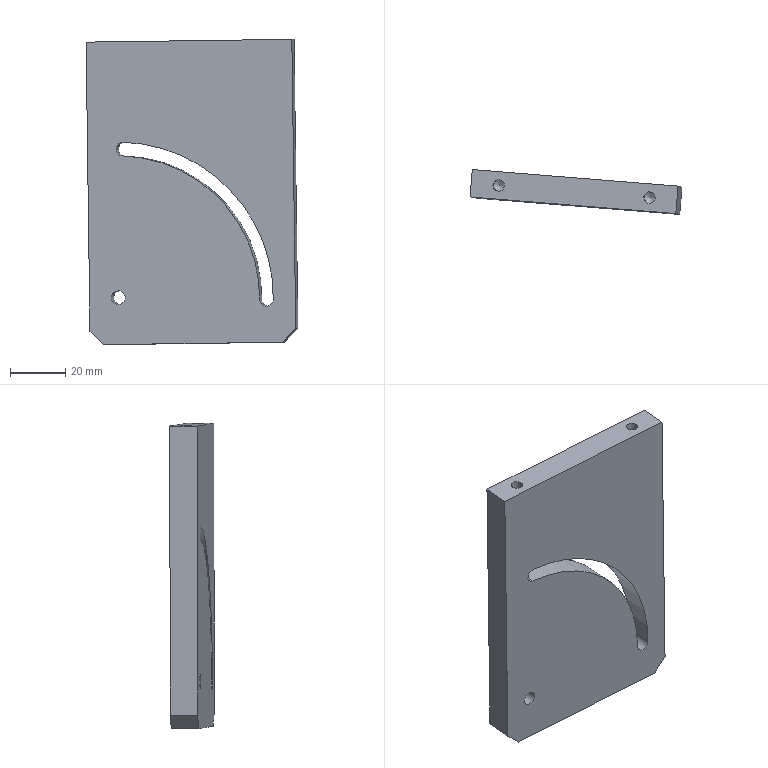Part | NX | 1 solid | 17 faces | box 76.959 x 16.139 x 110.936 mm | volume 77285 mm3 | plane 8 | cylinder 7 | cone 2 | commonest cylinder face diameters 5 x3 4.134 x2 103 x1 113 x1
STEP:
#1=CARTESIAN_POINT('',(751.636,682.46,909.631));
#2=VERTEX_POINT('',#1);
#3=CARTESIAN_POINT('',(752.438,692.427,909.627));
#4=VERTEX_POINT('',#3);
#5=CARTESIAN_POINT('',(751.636,682.46,909.631));
#6=DIRECTION('',(0.08022,0.9968,-0.0004004));
#7=VECTOR('',#6,1000.);
#8=LINE('',#5,#7);
#9=EDGE_CURVE('',#2,#4,#8,.T.);
#10=ORIENTED_EDGE('',*,*,#9,.F.);
#11=CARTESIAN_POINT('',(801.279,678.443,857.624));
#12=VERTEX_POINT('',#11);
#13=CARTESIAN_POINT('',(749.948,682.575,858.159));
#14=DIRECTION('',(-0.08022,-0.9968,0.0004004));
#15=DIRECTION('',(-0.01339,0.001479,0.9999));
#16=AXIS2_PLACEMENT_3D('',#13,#14,#15);
#17=CIRCLE('',#16,51.5);
#18=EDGE_CURVE('',#12,#2,#17,.T.);
#19=ORIENTED_EDGE('',*,*,#18,.F.);
#20=CARTESIAN_POINT('',(802.081,688.411,857.62));
#21=VERTEX_POINT('',#20);
#22=CARTESIAN_POINT('',(801.279,678.443,857.624));
#23=DIRECTION('',(-0.08022,-0.9968,0.0004004));
#24=VECTOR('',#23,1000.);
#25=LINE('',#22,#24);
#26=EDGE_CURVE('',#21,#12,#25,.T.);
#27=ORIENTED_EDGE('',*,*,#26,.F.);
#28=CARTESIAN_POINT('',(750.75,692.543,858.155));
#29=DIRECTION('',(0.08022,0.9968,-0.0004004));
#30=DIRECTION('',(-0.01339,0.001479,0.9999));
#31=AXIS2_PLACEMENT_3D('',#28,#29,#30);
#32=CIRCLE('',#31,51.5);
#33=EDGE_CURVE('',#4,#21,#32,.T.);
#34=ORIENTED_EDGE('',*,*,#33,.F.);
#35=EDGE_LOOP('',(#10,#19,#27,#34));
#36=FACE_BOUND('',#35,.T.);
#37=CARTESIAN_POINT('',(749.948,682.575,858.159));
#38=DIRECTION('',(0.08022,0.9968,-0.0004004));
#39=DIRECTION('',(-0.01339,0.001479,0.9999));
#40=AXIS2_PLACEMENT_3D('',#37,#38,#39);
#41=CYLINDRICAL_SURFACE('',#40,51.5);
#42=ADVANCED_FACE('',(#36),#41,.T.);
#43=CARTESIAN_POINT('',(751.8,682.449,914.628));
#44=VERTEX_POINT('',#43);
#45=CARTESIAN_POINT('',(751.718,682.454,912.13));
#46=DIRECTION('',(-0.08022,-0.9968,0.0004004));
#47=DIRECTION('',(-0.6979,0.05646,0.7139));
#48=AXIS2_PLACEMENT_3D('',#45,#46,#47);
#49=CIRCLE('',#48,2.5);
#50=EDGE_CURVE('',#44,#2,#49,.T.);
#51=ORIENTED_EDGE('',*,*,#50,.T.);
#52=ORIENTED_EDGE('',*,*,#9,.T.);
#53=CARTESIAN_POINT('',(752.602,692.416,914.624));
#54=VERTEX_POINT('',#53);
#55=CARTESIAN_POINT('',(752.52,692.422,912.126));
#56=DIRECTION('',(0.08022,0.9968,-0.0004004));
#57=DIRECTION('',(-0.7117,0.057,-0.7002));
#58=AXIS2_PLACEMENT_3D('',#55,#56,#57);
#59=CIRCLE('',#58,2.5);
#60=EDGE_CURVE('',#4,#54,#59,.T.);
#61=ORIENTED_EDGE('',*,*,#60,.T.);
#62=CARTESIAN_POINT('',(751.8,682.449,914.628));
#63=DIRECTION('',(-0.08022,-0.9968,0.0004004));
#64=VECTOR('',#63,1000.);
#65=LINE('',#62,#64);
#66=EDGE_CURVE('',#54,#44,#65,.T.);
#67=ORIENTED_EDGE('',*,*,#66,.T.);
#68=EDGE_LOOP('',(#51,#52,#61,#67));
#69=FACE_BOUND('',#68,.T.);
#70=CARTESIAN_POINT('',(751.718,682.454,912.13));
#71=DIRECTION('',(0.08022,0.9968,-0.0004004));
#72=DIRECTION('',(-0.6979,0.05646,0.7139));
#73=AXIS2_PLACEMENT_3D('',#70,#71,#72);
#74=CYLINDRICAL_SURFACE('',#73,2.5);
#75=ADVANCED_FACE('',(#69),#74,.F.);
#76=CARTESIAN_POINT('',(806.262,678.042,857.573));
#77=VERTEX_POINT('',#76);
#78=CARTESIAN_POINT('',(803.771,678.243,857.598));
#79=DIRECTION('',(-0.08022,-0.9968,0.0004004));
#80=DIRECTION('',(-0.7281,0.05832,-0.683));
#81=AXIS2_PLACEMENT_3D('',#78,#79,#80);
#82=CIRCLE('',#81,2.5);
#83=EDGE_CURVE('',#12,#77,#82,.T.);
#84=ORIENTED_EDGE('',*,*,#83,.T.);
#85=CARTESIAN_POINT('',(807.065,688.01,857.569));
#86=VERTEX_POINT('',#85);
#87=CARTESIAN_POINT('',(806.262,678.042,857.573));
#88=DIRECTION('',(0.08022,0.9968,-0.0004004));
#89=VECTOR('',#88,1000.);
#90=LINE('',#87,#89);
#91=EDGE_CURVE('',#77,#86,#90,.T.);
#92=ORIENTED_EDGE('',*,*,#91,.T.);
#93=CARTESIAN_POINT('',(804.573,688.211,857.594));
#94=DIRECTION('',(0.08022,0.9968,-0.0004004));
#95=DIRECTION('',(0.6808,-0.05509,-0.7304));
#96=AXIS2_PLACEMENT_3D('',#93,#94,#95);
#97=CIRCLE('',#96,2.5);
#98=EDGE_CURVE('',#86,#21,#97,.T.);
#99=ORIENTED_EDGE('',*,*,#98,.T.);
#100=ORIENTED_EDGE('',*,*,#26,.T.);
#101=EDGE_LOOP('',(#84,#92,#99,#100));
#102=FACE_BOUND('',#101,.T.);
#103=CARTESIAN_POINT('',(803.771,678.243,857.598));
#104=DIRECTION('',(0.08022,0.9968,-0.0004004));
#105=DIRECTION('',(0.6808,-0.05509,-0.7304));
#106=AXIS2_PLACEMENT_3D('',#103,#104,#105);
#107=CYLINDRICAL_SURFACE('',#106,2.5);
#108=ADVANCED_FACE('',(#102),#107,.F.);
#109=ORIENTED_EDGE('',*,*,#66,.F.);
#110=CARTESIAN_POINT('',(750.75,692.543,858.155));
#111=DIRECTION('',(-0.08022,-0.9968,0.0004004));
#112=DIRECTION('',(0.01339,-0.001479,-0.9999));
#113=AXIS2_PLACEMENT_3D('',#110,#111,#112);
#114=CIRCLE('',#113,56.5);
#115=EDGE_CURVE('',#86,#54,#114,.T.);
#116=ORIENTED_EDGE('',*,*,#115,.F.);
#117=ORIENTED_EDGE('',*,*,#91,.F.);
#118=CARTESIAN_POINT('',(749.948,682.575,858.159));
#119=DIRECTION('',(0.08022,0.9968,-0.0004004));
#120=DIRECTION('',(0.01339,-0.001479,-0.9999));
#121=AXIS2_PLACEMENT_3D('',#118,#119,#120);
#122=CIRCLE('',#121,56.5);
#123=EDGE_CURVE('',#44,#77,#122,.T.);
#124=ORIENTED_EDGE('',*,*,#123,.F.);
#125=EDGE_LOOP('',(#109,#116,#117,#124));
#126=FACE_BOUND('',#125,.T.);
#127=CARTESIAN_POINT('',(749.948,682.575,858.159));
#128=DIRECTION('',(0.08022,0.9968,-0.0004004));
#129=DIRECTION('',(0.01339,-0.001479,-0.9999));
#130=AXIS2_PLACEMENT_3D('',#127,#128,#129);
#131=CYLINDRICAL_SURFACE('',#130,56.5);
#132=ADVANCED_FACE('',(#126),#131,.F.);
#133=CARTESIAN_POINT('',(803.63,683.302,936.442));
#134=VERTEX_POINT('',#133);
#135=VERTEX_LOOP('',#134);
#136=FACE_BOUND('',#135,.T.);
#137=CARTESIAN_POINT('',(803.447,681.243,937.684));
#138=VERTEX_POINT('',#137);
#139=CARTESIAN_POINT('',(803.613,683.304,937.683));
#140=DIRECTION('',(-0.01339,0.001479,0.9999));
#141=DIRECTION('',(-0.08022,-0.9968,0.0004004));
#142=AXIS2_PLACEMENT_3D('',#139,#140,#141);
#143=CIRCLE('',#142,2.067);
#144=EDGE_CURVE('',#138,#138,#143,.T.);
#145=ORIENTED_EDGE('',*,*,#144,.T.);
#146=EDGE_LOOP('',(#145));
#147=FACE_BOUND('',#146,.T.);
#148=CARTESIAN_POINT('',(803.622,683.303,937.062));
#149=DIRECTION('',(-0.01339,0.001479,0.9999));
#150=DIRECTION('',(-0.08022,-0.9968,0.0004004));
#151=AXIS2_PLACEMENT_3D('',#148,#149,#150);
#152=CONICAL_SURFACE('',#151,1.034,1.03);
#153=ADVANCED_FACE('',(#136,#147),#152,.F.);
#154=ORIENTED_EDGE('',*,*,#144,.F.);
#155=EDGE_LOOP('',(#154));
#156=FACE_BOUND('',#155,.T.);
#157=CARTESIAN_POINT('',(803.257,681.264,951.883));
#158=VERTEX_POINT('',#157);
#159=CARTESIAN_POINT('',(803.423,683.325,951.882));
#160=DIRECTION('',(0.01339,-0.001479,-0.9999));
#161=DIRECTION('',(-0.08022,-0.9968,0.0004004));
#162=AXIS2_PLACEMENT_3D('',#159,#160,#161);
#163=CIRCLE('',#162,2.067);
#164=EDGE_CURVE('',#158,#158,#163,.T.);
#165=ORIENTED_EDGE('',*,*,#164,.F.);
#166=EDGE_LOOP('',(#165));
#167=FACE_BOUND('',#166,.T.);
#168=CARTESIAN_POINT('',(803.518,683.314,944.783));
#169=DIRECTION('',(-0.01339,0.001479,0.9999));
#170=DIRECTION('',(-0.08022,-0.9968,0.0004004));
#171=AXIS2_PLACEMENT_3D('',#168,#169,#170);
#172=CYLINDRICAL_SURFACE('',#171,2.067);
#173=ADVANCED_FACE('',(#156,#167),#172,.F.);
#174=CARTESIAN_POINT('',(748.812,687.714,935.701));
#175=VERTEX_POINT('',#174);
#176=VERTEX_LOOP('',#175);
#177=FACE_BOUND('',#176,.T.);
#178=CARTESIAN_POINT('',(748.63,685.655,936.944));
#179=VERTEX_POINT('',#178);
#180=CARTESIAN_POINT('',(748.796,687.715,936.943));
#181=DIRECTION('',(-0.01339,0.001479,0.9999));
#182=DIRECTION('',(-0.08022,-0.9968,0.0004004));
#183=AXIS2_PLACEMENT_3D('',#180,#181,#182);
#184=CIRCLE('',#183,2.067);
#185=EDGE_CURVE('',#179,#179,#184,.T.);
#186=ORIENTED_EDGE('',*,*,#185,.T.);
#187=EDGE_LOOP('',(#186));
#188=FACE_BOUND('',#187,.T.);
#189=CARTESIAN_POINT('',(748.804,687.715,936.322));
#190=DIRECTION('',(-0.01339,0.001479,0.9999));
#191=DIRECTION('',(-0.08022,-0.9968,0.0004004));
#192=AXIS2_PLACEMENT_3D('',#189,#190,#191);
#193=CONICAL_SURFACE('',#192,1.034,1.03);
#194=ADVANCED_FACE('',(#177,#188),#193,.F.);
#195=ORIENTED_EDGE('',*,*,#185,.F.);
#196=EDGE_LOOP('',(#195));
#197=FACE_BOUND('',#196,.T.);
#198=CARTESIAN_POINT('',(748.44,685.676,951.143));
#199=VERTEX_POINT('',#198);
#200=CARTESIAN_POINT('',(748.605,687.736,951.142));
#201=DIRECTION('',(0.01339,-0.001479,-0.9999));
#202=DIRECTION('',(-0.08022,-0.9968,0.0004004));
#203=AXIS2_PLACEMENT_3D('',#200,#201,#202);
#204=CIRCLE('',#203,2.067);
#205=EDGE_CURVE('',#199,#199,#204,.T.);
#206=ORIENTED_EDGE('',*,*,#205,.F.);
#207=EDGE_LOOP('',(#206));
#208=FACE_BOUND('',#207,.T.);
#209=CARTESIAN_POINT('',(748.7,687.726,944.042));
#210=DIRECTION('',(-0.01339,0.001479,0.9999));
#211=DIRECTION('',(-0.08022,-0.9968,0.0004004));
#212=AXIS2_PLACEMENT_3D('',#209,#210,#211);
#213=CYLINDRICAL_SURFACE('',#212,2.067);
#214=ADVANCED_FACE('',(#197,#208),#213,.F.);
#215=CARTESIAN_POINT('',(750.783,692.539,855.655));
#216=VERTEX_POINT('',#215);
#217=CARTESIAN_POINT('',(750.75,692.543,858.155));
#218=DIRECTION('',(-0.08022,-0.9968,0.0004004));
#219=DIRECTION('',(0.01339,-0.001479,-0.9999));
#220=AXIS2_PLACEMENT_3D('',#217,#218,#219);
#221=CIRCLE('',#220,2.5);
#222=EDGE_CURVE('',#216,#216,#221,.T.);
#223=ORIENTED_EDGE('',*,*,#222,.F.);
#224=EDGE_LOOP('',(#223));
#225=FACE_BOUND('',#224,.T.);
#226=CARTESIAN_POINT('',(749.981,682.571,855.659));
#227=VERTEX_POINT('',#226);
#228=CARTESIAN_POINT('',(749.948,682.575,858.159));
#229=DIRECTION('',(0.08022,0.9968,-0.0004004));
#230=DIRECTION('',(0.01339,-0.001479,-0.9999));
#231=AXIS2_PLACEMENT_3D('',#228,#229,#230);
#232=CIRCLE('',#231,2.5);
#233=EDGE_CURVE('',#227,#227,#232,.T.);
#234=ORIENTED_EDGE('',*,*,#233,.F.);
#235=EDGE_LOOP('',(#234));
#236=FACE_BOUND('',#235,.T.);
#237=CARTESIAN_POINT('',(760.658,815.655,858.105));
#238=DIRECTION('',(-0.08022,-0.9968,0.0004004));
#239=DIRECTION('',(0.01339,-0.001479,-0.9999));
#240=AXIS2_PLACEMENT_3D('',#237,#238,#239);
#241=CYLINDRICAL_SURFACE('',#240,2.5);
#242=ADVANCED_FACE('',(#225,#236),#241,.F.);
#243=CARTESIAN_POINT('',(810.28,687.745,841.957));
#244=VERTEX_POINT('',#243);
#245=CARTESIAN_POINT('',(815.197,687.351,847.024));
#246=VERTEX_POINT('',#245);
#247=CARTESIAN_POINT('',(817.041,687.204,848.924));
#248=DIRECTION('',(0.6953,-0.05567,0.7166));
#249=VECTOR('',#248,1000.);
#250=LINE('',#247,#249);
#251=EDGE_CURVE('',#244,#246,#250,.T.);
#252=ORIENTED_EDGE('',*,*,#251,.T.);
#253=CARTESIAN_POINT('',(814.395,677.383,847.028));
#254=VERTEX_POINT('',#253);
#255=CARTESIAN_POINT('',(814.395,677.383,847.028));
#256=DIRECTION('',(-0.08022,-0.9968,0.0004004));
#257=VECTOR('',#256,1000.);
#258=LINE('',#255,#257);
#259=EDGE_CURVE('',#246,#254,#258,.T.);
#260=ORIENTED_EDGE('',*,*,#259,.T.);
#261=CARTESIAN_POINT('',(809.478,677.777,841.961));
#262=VERTEX_POINT('',#261);
#263=CARTESIAN_POINT('',(816.238,677.236,848.928));
#264=DIRECTION('',(-0.6953,0.05567,-0.7166));
#265=VECTOR('',#264,1000.);
#266=LINE('',#263,#265);
#267=EDGE_CURVE('',#254,#262,#266,.T.);
#268=ORIENTED_EDGE('',*,*,#267,.T.);
#269=CARTESIAN_POINT('',(809.478,677.777,841.961));
#270=DIRECTION('',(0.08022,0.9968,-0.0004004));
#271=VECTOR('',#270,1000.);
#272=LINE('',#269,#271);
#273=EDGE_CURVE('',#262,#244,#272,.T.);
#274=ORIENTED_EDGE('',*,*,#273,.T.);
#275=EDGE_LOOP('',(#252,#260,#268,#274));
#276=FACE_BOUND('',#275,.T.);
#277=CARTESIAN_POINT('',(811.936,677.58,844.495));
#278=DIRECTION('',(0.7142,-0.05776,-0.6975));
#279=DIRECTION('',(0.08022,0.9968,-0.0004004));
#280=AXIS2_PLACEMENT_3D('',#277,#278,#279);
#281=PLANE('',#280);
#282=ADVANCED_FACE('',(#276),#281,.T.);
#283=ORIENTED_EDGE('',*,*,#273,.F.);
#284=CARTESIAN_POINT('',(744.693,682.991,841.086));
#285=VERTEX_POINT('',#284);
#286=CARTESIAN_POINT('',(814.462,677.376,842.029));
#287=DIRECTION('',(-0.9967,0.08021,-0.01346));
#288=VECTOR('',#287,1000.);
#289=LINE('',#286,#288);
#290=EDGE_CURVE('',#262,#285,#289,.T.);
#291=ORIENTED_EDGE('',*,*,#290,.T.);
#292=CARTESIAN_POINT('',(745.496,692.959,841.082));
#293=VERTEX_POINT('',#292);
#294=CARTESIAN_POINT('',(744.693,682.991,841.086));
#295=DIRECTION('',(-0.08022,-0.9968,0.0004004));
#296=VECTOR('',#295,1000.);
#297=LINE('',#294,#296);
#298=EDGE_CURVE('',#293,#285,#297,.T.);
#299=ORIENTED_EDGE('',*,*,#298,.F.);
#300=CARTESIAN_POINT('',(815.264,687.344,842.025));
#301=DIRECTION('',(-0.9967,0.08021,-0.01346));
#302=VECTOR('',#301,1000.);
#303=LINE('',#300,#302);
#304=EDGE_CURVE('',#244,#293,#303,.T.);
#305=ORIENTED_EDGE('',*,*,#304,.F.);
#306=EDGE_LOOP('',(#283,#291,#299,#305));
#307=FACE_BOUND('',#306,.T.);
#308=CARTESIAN_POINT('',(814.462,677.376,842.029));
#309=DIRECTION('',(0.01339,-0.001479,-0.9999));
#310=DIRECTION('',(-0.9967,0.08021,-0.01346));
#311=AXIS2_PLACEMENT_3D('',#308,#309,#310);
#312=PLANE('',#311);
#313=ADVANCED_FACE('',(#307),#312,.T.);
#314=ORIENTED_EDGE('',*,*,#267,.F.);
#315=CARTESIAN_POINT('',(812.989,677.539,952.019));
#316=VERTEX_POINT('',#315);
#317=CARTESIAN_POINT('',(812.989,677.539,952.019));
#318=DIRECTION('',(0.01339,-0.001479,-0.9999));
#319=VECTOR('',#318,1000.);
#320=LINE('',#317,#319);
#321=EDGE_CURVE('',#316,#254,#320,.T.);
#322=ORIENTED_EDGE('',*,*,#321,.F.);
#323=CARTESIAN_POINT('',(738.237,683.555,951.009));
#324=VERTEX_POINT('',#323);
#325=CARTESIAN_POINT('',(738.237,683.555,951.009));
#326=DIRECTION('',(0.9967,-0.08021,0.01346));
#327=VECTOR('',#326,1000.);
#328=LINE('',#325,#327);
#329=EDGE_CURVE('',#324,#316,#328,.T.);
#330=ORIENTED_EDGE('',*,*,#329,.F.);
#331=CARTESIAN_POINT('',(739.643,683.399,846.019));
#332=VERTEX_POINT('',#331);
#333=CARTESIAN_POINT('',(739.71,683.392,841.019));
#334=DIRECTION('',(-0.01339,0.001479,0.9999));
#335=VECTOR('',#334,1000.);
#336=LINE('',#333,#335);
#337=EDGE_CURVE('',#332,#324,#336,.T.);
#338=ORIENTED_EDGE('',*,*,#337,.F.);
#339=CARTESIAN_POINT('',(737.749,683.553,847.868));
#340=DIRECTION('',(-0.7142,0.05776,0.6975));
#341=VECTOR('',#340,1000.);
#342=LINE('',#339,#341);
#343=EDGE_CURVE('',#285,#332,#342,.T.);
#344=ORIENTED_EDGE('',*,*,#343,.F.);
#345=ORIENTED_EDGE('',*,*,#290,.F.);
#346=EDGE_LOOP('',(#314,#322,#330,#338,#344,#345));
#347=FACE_BOUND('',#346,.T.);
#348=ORIENTED_EDGE('',*,*,#18,.T.);
#349=ORIENTED_EDGE('',*,*,#50,.F.);
#350=ORIENTED_EDGE('',*,*,#123,.T.);
#351=ORIENTED_EDGE('',*,*,#83,.F.);
#352=EDGE_LOOP('',(#348,#349,#350,#351));
#353=FACE_BOUND('',#352,.T.);
#354=ORIENTED_EDGE('',*,*,#233,.T.);
#355=EDGE_LOOP('',(#354));
#356=FACE_BOUND('',#355,.T.);
#357=CARTESIAN_POINT('',(776.349,680.465,896.519));
#358=DIRECTION('',(0.08022,0.9968,-0.0004004));
#359=DIRECTION('',(-0.01339,0.001479,0.9999));
#360=AXIS2_PLACEMENT_3D('',#357,#358,#359);
#361=PLANE('',#360);
#362=ADVANCED_FACE('',(#347,#353,#356),#361,.F.);
#363=CARTESIAN_POINT('',(740.445,693.367,846.015));
#364=VERTEX_POINT('',#363);
#365=CARTESIAN_POINT('',(738.551,693.52,847.864));
#366=DIRECTION('',(0.7142,-0.05776,-0.6975));
#367=VECTOR('',#366,1000.);
#368=LINE('',#365,#367);
#369=EDGE_CURVE('',#364,#293,#368,.T.);
#370=ORIENTED_EDGE('',*,*,#369,.T.);
#371=ORIENTED_EDGE('',*,*,#298,.T.);
#372=ORIENTED_EDGE('',*,*,#343,.T.);
#373=CARTESIAN_POINT('',(739.643,683.399,846.019));
#374=DIRECTION('',(0.08022,0.9968,-0.0004004));
#375=VECTOR('',#374,1000.);
#376=LINE('',#373,#375);
#377=EDGE_CURVE('',#332,#364,#376,.T.);
#378=ORIENTED_EDGE('',*,*,#377,.T.);
#379=EDGE_LOOP('',(#370,#371,#372,#378));
#380=FACE_BOUND('',#379,.T.);
#381=CARTESIAN_POINT('',(742.168,683.195,843.552));
#382=DIRECTION('',(-0.6953,0.05567,-0.7166));
#383=DIRECTION('',(0.08022,0.9968,-0.0004004));
#384=AXIS2_PLACEMENT_3D('',#381,#382,#383);
#385=PLANE('',#384);
#386=ADVANCED_FACE('',(#380),#385,.T.);
#387=ORIENTED_EDGE('',*,*,#377,.F.);
#388=ORIENTED_EDGE('',*,*,#337,.T.);
#389=CARTESIAN_POINT('',(739.04,693.522,951.005));
#390=VERTEX_POINT('',#389);
#391=CARTESIAN_POINT('',(738.237,683.555,951.009));
#392=DIRECTION('',(0.08022,0.9968,-0.0004004));
#393=VECTOR('',#392,1000.);
#394=LINE('',#391,#393);
#395=EDGE_CURVE('',#324,#390,#394,.T.);
#396=ORIENTED_EDGE('',*,*,#395,.T.);
#397=CARTESIAN_POINT('',(740.512,693.36,841.015));
#398=DIRECTION('',(-0.01339,0.001479,0.9999));
#399=VECTOR('',#398,1000.);
#400=LINE('',#397,#399);
#401=EDGE_CURVE('',#364,#390,#400,.T.);
#402=ORIENTED_EDGE('',*,*,#401,.F.);
#403=EDGE_LOOP('',(#387,#388,#396,#402));
#404=FACE_BOUND('',#403,.T.);
#405=CARTESIAN_POINT('',(739.71,683.392,841.019));
#406=DIRECTION('',(-0.9967,0.08021,-0.01346));
#407=DIRECTION('',(-0.01339,0.001479,0.9999));
#408=AXIS2_PLACEMENT_3D('',#405,#406,#407);
#409=PLANE('',#408);
#410=ADVANCED_FACE('',(#404),#409,.T.);
#411=ORIENTED_EDGE('',*,*,#259,.F.);
#412=CARTESIAN_POINT('',(813.791,687.507,952.015));
#413=VERTEX_POINT('',#412);
#414=CARTESIAN_POINT('',(813.791,687.507,952.015));
#415=DIRECTION('',(0.01339,-0.001479,-0.9999));
#416=VECTOR('',#415,1000.);
#417=LINE('',#414,#416);
#418=EDGE_CURVE('',#413,#246,#417,.T.);
#419=ORIENTED_EDGE('',*,*,#418,.F.);
#420=CARTESIAN_POINT('',(812.989,677.539,952.019));
#421=DIRECTION('',(0.08022,0.9968,-0.0004004));
#422=VECTOR('',#421,1000.);
#423=LINE('',#420,#422);
#424=EDGE_CURVE('',#316,#413,#423,.T.);
#425=ORIENTED_EDGE('',*,*,#424,.F.);
#426=ORIENTED_EDGE('',*,*,#321,.T.);
#427=EDGE_LOOP('',(#411,#419,#425,#426));
#428=FACE_BOUND('',#427,.T.);
#429=CARTESIAN_POINT('',(812.989,677.539,952.019));
#430=DIRECTION('',(0.9967,-0.08021,0.01346));
#431=DIRECTION('',(0.01339,-0.001479,-0.9999));
#432=AXIS2_PLACEMENT_3D('',#429,#430,#431);
#433=PLANE('',#432);
#434=ADVANCED_FACE('',(#428),#433,.T.);
#435=ORIENTED_EDGE('',*,*,#329,.T.);
#436=ORIENTED_EDGE('',*,*,#424,.T.);
#437=CARTESIAN_POINT('',(739.04,693.522,951.005));
#438=DIRECTION('',(0.9967,-0.08021,0.01346));
#439=VECTOR('',#438,1000.);
#440=LINE('',#437,#439);
#441=EDGE_CURVE('',#390,#413,#440,.T.);
#442=ORIENTED_EDGE('',*,*,#441,.F.);
#443=ORIENTED_EDGE('',*,*,#395,.F.);
#444=EDGE_LOOP('',(#435,#436,#442,#443));
#445=FACE_BOUND('',#444,.T.);
#446=ORIENTED_EDGE('',*,*,#164,.T.);
#447=EDGE_LOOP('',(#446));
#448=FACE_BOUND('',#447,.T.);
#449=ORIENTED_EDGE('',*,*,#205,.T.);
#450=EDGE_LOOP('',(#449));
#451=FACE_BOUND('',#450,.T.);
#452=CARTESIAN_POINT('',(738.237,683.555,951.009));
#453=DIRECTION('',(-0.01339,0.001479,0.9999));
#454=DIRECTION('',(0.9967,-0.08021,0.01346));
#455=AXIS2_PLACEMENT_3D('',#452,#453,#454);
#456=PLANE('',#455);
#457=ADVANCED_FACE('',(#445,#448,#451),#456,.T.);
#458=ORIENTED_EDGE('',*,*,#251,.F.);
#459=ORIENTED_EDGE('',*,*,#304,.T.);
#460=ORIENTED_EDGE('',*,*,#369,.F.);
#461=ORIENTED_EDGE('',*,*,#401,.T.);
#462=ORIENTED_EDGE('',*,*,#441,.T.);
#463=ORIENTED_EDGE('',*,*,#418,.T.);
#464=EDGE_LOOP('',(#458,#459,#460,#461,#462,#463));
#465=FACE_BOUND('',#464,.T.);
#466=ORIENTED_EDGE('',*,*,#33,.T.);
#467=ORIENTED_EDGE('',*,*,#98,.F.);
#468=ORIENTED_EDGE('',*,*,#115,.T.);
#469=ORIENTED_EDGE('',*,*,#60,.F.);
#470=EDGE_LOOP('',(#466,#467,#468,#469));
#471=FACE_BOUND('',#470,.T.);
#472=ORIENTED_EDGE('',*,*,#222,.T.);
#473=EDGE_LOOP('',(#472));
#474=FACE_BOUND('',#473,.T.);
#475=CARTESIAN_POINT('',(777.152,690.433,896.515));
#476=DIRECTION('',(0.08022,0.9968,-0.0004004));
#477=DIRECTION('',(-0.01339,0.001479,0.9999));
#478=AXIS2_PLACEMENT_3D('',#475,#476,#477);
#479=PLANE('',#478);
#480=ADVANCED_FACE('',(#465,#471,#474),#479,.T.);
#481=CLOSED_SHELL('',(#42,#75,#108,#132,#153,#173,#194,#214,#242,#282,#313,#362,#386,#410,#434,#457,#480));
#482=MANIFOLD_SOLID_BREP('',#481);
#483=(LENGTH_UNIT()NAMED_UNIT(*)SI_UNIT(.MILLI.,.METRE.));
#484=UNCERTAINTY_MEASURE_WITH_UNIT(LENGTH_MEASURE(0.00001),#483,'','');
#485=(NAMED_UNIT(*)PLANE_ANGLE_UNIT()SI_UNIT($,.RADIAN.));
#486=(NAMED_UNIT(*)SI_UNIT($,.STERADIAN.)SOLID_ANGLE_UNIT());
#487=(GEOMETRIC_REPRESENTATION_CONTEXT(3)GLOBAL_UNCERTAINTY_ASSIGNED_CONTEXT((#484))GLOBAL_UNIT_ASSIGNED_CONTEXT((#483,#485,#486))REPRESENTATION_CONTEXT('',''));
#488=ADVANCED_BREP_SHAPE_REPRESENTATION('',(#482),#487);